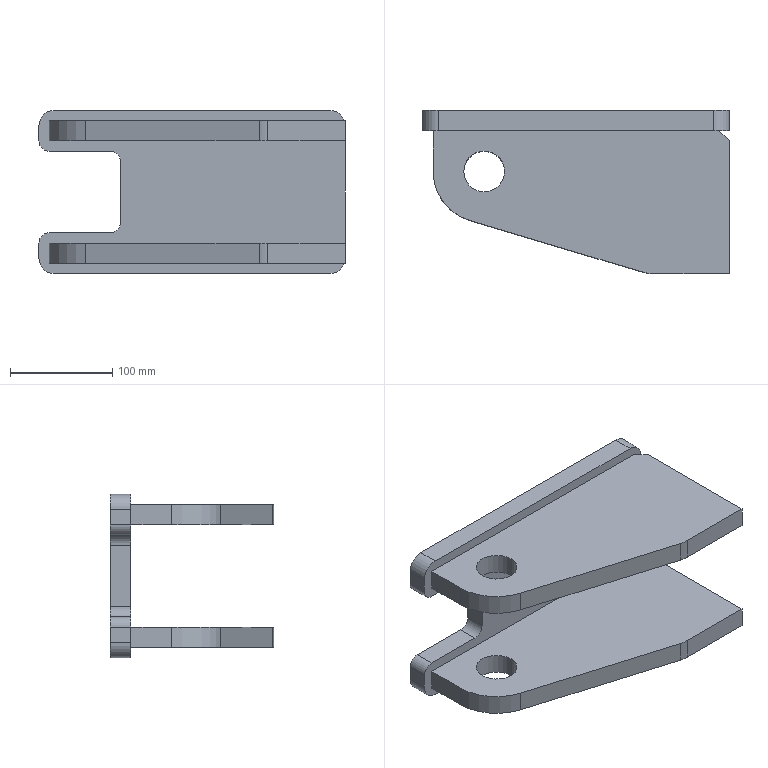Part | SolidWorks | features BaseBody 3 | 3 solids | 42 faces | box 300 x 160 x 160 mm | volume 2125789 mm3 | plane 26 | cylinder 16 | commonest cylinder face diameters 20 x4 30 x4 40 x4 60 x2 100 x2
STEP:
#1=CARTESIAN_POINT('',(-150.,-10.,-65.));
#2=VERTEX_POINT('',#1);
#3=CARTESIAN_POINT('',(-150.,-10.,-50.));
#4=VERTEX_POINT('',#3);
#5=CARTESIAN_POINT('',(-150.,-10.,-65.));
#6=DIRECTION('',(0.,0.,1.));
#7=VECTOR('',#6,1000.);
#8=LINE('',#5,#7);
#9=EDGE_CURVE('',#2,#4,#8,.T.);
#10=ORIENTED_EDGE('',*,*,#9,.T.);
#11=CARTESIAN_POINT('',(-150.,10.,-50.));
#12=VERTEX_POINT('',#11);
#13=CARTESIAN_POINT('',(-150.,10.,-50.));
#14=DIRECTION('',(0.,1.,0.));
#15=VECTOR('',#14,1000.);
#16=LINE('',#13,#15);
#17=EDGE_CURVE('',#4,#12,#16,.T.);
#18=ORIENTED_EDGE('',*,*,#17,.T.);
#19=CARTESIAN_POINT('',(-150.,10.,-65.));
#20=VERTEX_POINT('',#19);
#21=CARTESIAN_POINT('',(-150.,10.,-65.));
#22=DIRECTION('',(0.,0.,1.));
#23=VECTOR('',#22,1000.);
#24=LINE('',#21,#23);
#25=EDGE_CURVE('',#20,#12,#24,.T.);
#26=ORIENTED_EDGE('',*,*,#25,.F.);
#27=CARTESIAN_POINT('',(-150.,10.,-65.));
#28=DIRECTION('',(0.,-1.,0.));
#29=VECTOR('',#28,1000.);
#30=LINE('',#27,#29);
#31=EDGE_CURVE('',#20,#2,#30,.T.);
#32=ORIENTED_EDGE('',*,*,#31,.T.);
#33=EDGE_LOOP('',(#10,#18,#26,#32));
#34=FACE_OUTER_BOUND('',#33,.T.);
#35=CARTESIAN_POINT('',(-150.,10.,-65.));
#36=DIRECTION('',(1.,0.,0.));
#37=DIRECTION('',(0.,0.,-1.));
#38=AXIS2_PLACEMENT_3D('',#35,#36,#37);
#39=PLANE('',#38);
#40=ADVANCED_FACE('',(#34),#39,.F.);
#41=CARTESIAN_POINT('',(-150.,-10.,65.));
#42=VERTEX_POINT('',#41);
#43=CARTESIAN_POINT('',(-135.,-10.,80.));
#44=VERTEX_POINT('',#43);
#45=CARTESIAN_POINT('',(-135.,-10.,65.));
#46=DIRECTION('',(0.,1.,0.));
#47=DIRECTION('',(0.,0.,1.));
#48=AXIS2_PLACEMENT_3D('',#45,#46,#47);
#49=CIRCLE('',#48,15.);
#50=EDGE_CURVE('',#42,#44,#49,.T.);
#51=ORIENTED_EDGE('',*,*,#50,.T.);
#52=CARTESIAN_POINT('',(-135.,10.,80.));
#53=VERTEX_POINT('',#52);
#54=CARTESIAN_POINT('',(-135.,10.,80.));
#55=DIRECTION('',(0.,-1.,0.));
#56=VECTOR('',#55,1000.);
#57=LINE('',#54,#56);
#58=EDGE_CURVE('',#53,#44,#57,.T.);
#59=ORIENTED_EDGE('',*,*,#58,.F.);
#60=CARTESIAN_POINT('',(-150.,10.,65.));
#61=VERTEX_POINT('',#60);
#62=CARTESIAN_POINT('',(-135.,10.,65.));
#63=DIRECTION('',(0.,1.,0.));
#64=DIRECTION('',(0.,0.,1.));
#65=AXIS2_PLACEMENT_3D('',#62,#63,#64);
#66=CIRCLE('',#65,15.);
#67=EDGE_CURVE('',#61,#53,#66,.T.);
#68=ORIENTED_EDGE('',*,*,#67,.F.);
#69=CARTESIAN_POINT('',(-150.,10.,65.));
#70=DIRECTION('',(0.,-1.,0.));
#71=VECTOR('',#70,1000.);
#72=LINE('',#69,#71);
#73=EDGE_CURVE('',#61,#42,#72,.T.);
#74=ORIENTED_EDGE('',*,*,#73,.T.);
#75=EDGE_LOOP('',(#51,#59,#68,#74));
#76=FACE_OUTER_BOUND('',#75,.T.);
#77=CARTESIAN_POINT('',(-135.,10.,65.));
#78=DIRECTION('',(0.,-1.,0.));
#79=DIRECTION('',(0.,0.,-1.));
#80=AXIS2_PLACEMENT_3D('',#77,#78,#79);
#81=CYLINDRICAL_SURFACE('',#80,15.);
#82=ADVANCED_FACE('',(#76),#81,.T.);
#83=CARTESIAN_POINT('',(135.,-10.,80.));
#84=VERTEX_POINT('',#83);
#85=CARTESIAN_POINT('',(-135.,-10.,80.));
#86=DIRECTION('',(1.,0.,0.));
#87=VECTOR('',#86,1000.);
#88=LINE('',#85,#87);
#89=EDGE_CURVE('',#44,#84,#88,.T.);
#90=ORIENTED_EDGE('',*,*,#89,.T.);
#91=CARTESIAN_POINT('',(135.,10.,80.));
#92=VERTEX_POINT('',#91);
#93=CARTESIAN_POINT('',(135.,10.,80.));
#94=DIRECTION('',(0.,-1.,0.));
#95=VECTOR('',#94,1000.);
#96=LINE('',#93,#95);
#97=EDGE_CURVE('',#92,#84,#96,.T.);
#98=ORIENTED_EDGE('',*,*,#97,.F.);
#99=CARTESIAN_POINT('',(-135.,10.,80.));
#100=DIRECTION('',(1.,0.,0.));
#101=VECTOR('',#100,1000.);
#102=LINE('',#99,#101);
#103=EDGE_CURVE('',#53,#92,#102,.T.);
#104=ORIENTED_EDGE('',*,*,#103,.F.);
#105=ORIENTED_EDGE('',*,*,#58,.T.);
#106=EDGE_LOOP('',(#90,#98,#104,#105));
#107=FACE_OUTER_BOUND('',#106,.T.);
#108=CARTESIAN_POINT('',(-135.,10.,80.));
#109=DIRECTION('',(0.,0.,-1.));
#110=DIRECTION('',(-1.,0.,0.));
#111=AXIS2_PLACEMENT_3D('',#108,#109,#110);
#112=PLANE('',#111);
#113=ADVANCED_FACE('',(#107),#112,.F.);
#114=CARTESIAN_POINT('',(150.,-10.,65.));
#115=VERTEX_POINT('',#114);
#116=CARTESIAN_POINT('',(135.,-10.,65.));
#117=DIRECTION('',(0.,1.,0.));
#118=DIRECTION('',(0.,0.,1.));
#119=AXIS2_PLACEMENT_3D('',#116,#117,#118);
#120=CIRCLE('',#119,15.);
#121=EDGE_CURVE('',#84,#115,#120,.T.);
#122=ORIENTED_EDGE('',*,*,#121,.T.);
#123=CARTESIAN_POINT('',(150.,10.,65.));
#124=VERTEX_POINT('',#123);
#125=CARTESIAN_POINT('',(150.,10.,65.));
#126=DIRECTION('',(0.,-1.,0.));
#127=VECTOR('',#126,1000.);
#128=LINE('',#125,#127);
#129=EDGE_CURVE('',#124,#115,#128,.T.);
#130=ORIENTED_EDGE('',*,*,#129,.F.);
#131=CARTESIAN_POINT('',(135.,10.,65.));
#132=DIRECTION('',(0.,1.,0.));
#133=DIRECTION('',(0.,0.,1.));
#134=AXIS2_PLACEMENT_3D('',#131,#132,#133);
#135=CIRCLE('',#134,15.);
#136=EDGE_CURVE('',#92,#124,#135,.T.);
#137=ORIENTED_EDGE('',*,*,#136,.F.);
#138=ORIENTED_EDGE('',*,*,#97,.T.);
#139=EDGE_LOOP('',(#122,#130,#137,#138));
#140=FACE_OUTER_BOUND('',#139,.T.);
#141=CARTESIAN_POINT('',(135.,10.,65.));
#142=DIRECTION('',(0.,-1.,0.));
#143=DIRECTION('',(0.,0.,-1.));
#144=AXIS2_PLACEMENT_3D('',#141,#142,#143);
#145=CYLINDRICAL_SURFACE('',#144,15.);
#146=ADVANCED_FACE('',(#140),#145,.T.);
#147=CARTESIAN_POINT('',(150.,-10.,-65.));
#148=VERTEX_POINT('',#147);
#149=CARTESIAN_POINT('',(150.,-10.,-65.));
#150=DIRECTION('',(0.,0.,-1.));
#151=VECTOR('',#150,1000.);
#152=LINE('',#149,#151);
#153=EDGE_CURVE('',#115,#148,#152,.T.);
#154=ORIENTED_EDGE('',*,*,#153,.T.);
#155=CARTESIAN_POINT('',(150.,10.,-65.));
#156=VERTEX_POINT('',#155);
#157=CARTESIAN_POINT('',(150.,10.,-65.));
#158=DIRECTION('',(0.,-1.,0.));
#159=VECTOR('',#158,1000.);
#160=LINE('',#157,#159);
#161=EDGE_CURVE('',#156,#148,#160,.T.);
#162=ORIENTED_EDGE('',*,*,#161,.F.);
#163=CARTESIAN_POINT('',(150.,10.,-65.));
#164=DIRECTION('',(0.,0.,-1.));
#165=VECTOR('',#164,1000.);
#166=LINE('',#163,#165);
#167=EDGE_CURVE('',#124,#156,#166,.T.);
#168=ORIENTED_EDGE('',*,*,#167,.F.);
#169=ORIENTED_EDGE('',*,*,#129,.T.);
#170=EDGE_LOOP('',(#154,#162,#168,#169));
#171=FACE_OUTER_BOUND('',#170,.T.);
#172=CARTESIAN_POINT('',(150.,10.,-65.));
#173=DIRECTION('',(-1.,0.,0.));
#174=DIRECTION('',(0.,0.,1.));
#175=AXIS2_PLACEMENT_3D('',#172,#173,#174);
#176=PLANE('',#175);
#177=ADVANCED_FACE('',(#171),#176,.F.);
#178=CARTESIAN_POINT('',(135.,-10.,-80.));
#179=VERTEX_POINT('',#178);
#180=CARTESIAN_POINT('',(135.,-10.,-65.));
#181=DIRECTION('',(0.,1.,0.));
#182=DIRECTION('',(0.,0.,-1.));
#183=AXIS2_PLACEMENT_3D('',#180,#181,#182);
#184=CIRCLE('',#183,15.);
#185=EDGE_CURVE('',#148,#179,#184,.T.);
#186=ORIENTED_EDGE('',*,*,#185,.T.);
#187=CARTESIAN_POINT('',(135.,10.,-80.));
#188=VERTEX_POINT('',#187);
#189=CARTESIAN_POINT('',(135.,10.,-80.));
#190=DIRECTION('',(0.,-1.,0.));
#191=VECTOR('',#190,1000.);
#192=LINE('',#189,#191);
#193=EDGE_CURVE('',#188,#179,#192,.T.);
#194=ORIENTED_EDGE('',*,*,#193,.F.);
#195=CARTESIAN_POINT('',(135.,10.,-65.));
#196=DIRECTION('',(0.,1.,0.));
#197=DIRECTION('',(0.,0.,-1.));
#198=AXIS2_PLACEMENT_3D('',#195,#196,#197);
#199=CIRCLE('',#198,15.);
#200=EDGE_CURVE('',#156,#188,#199,.T.);
#201=ORIENTED_EDGE('',*,*,#200,.F.);
#202=ORIENTED_EDGE('',*,*,#161,.T.);
#203=EDGE_LOOP('',(#186,#194,#201,#202));
#204=FACE_OUTER_BOUND('',#203,.T.);
#205=CARTESIAN_POINT('',(135.,10.,-65.));
#206=DIRECTION('',(0.,-1.,0.));
#207=DIRECTION('',(0.,0.,-1.));
#208=AXIS2_PLACEMENT_3D('',#205,#206,#207);
#209=CYLINDRICAL_SURFACE('',#208,15.);
#210=ADVANCED_FACE('',(#204),#209,.T.);
#211=CARTESIAN_POINT('',(-135.,-10.,-80.));
#212=VERTEX_POINT('',#211);
#213=CARTESIAN_POINT('',(-135.,-10.,-80.));
#214=DIRECTION('',(-1.,0.,0.));
#215=VECTOR('',#214,1000.);
#216=LINE('',#213,#215);
#217=EDGE_CURVE('',#179,#212,#216,.T.);
#218=ORIENTED_EDGE('',*,*,#217,.T.);
#219=CARTESIAN_POINT('',(-135.,10.,-80.));
#220=VERTEX_POINT('',#219);
#221=CARTESIAN_POINT('',(-135.,10.,-80.));
#222=DIRECTION('',(0.,-1.,0.));
#223=VECTOR('',#222,1000.);
#224=LINE('',#221,#223);
#225=EDGE_CURVE('',#220,#212,#224,.T.);
#226=ORIENTED_EDGE('',*,*,#225,.F.);
#227=CARTESIAN_POINT('',(-135.,10.,-80.));
#228=DIRECTION('',(-1.,0.,0.));
#229=VECTOR('',#228,1000.);
#230=LINE('',#227,#229);
#231=EDGE_CURVE('',#188,#220,#230,.T.);
#232=ORIENTED_EDGE('',*,*,#231,.F.);
#233=ORIENTED_EDGE('',*,*,#193,.T.);
#234=EDGE_LOOP('',(#218,#226,#232,#233));
#235=FACE_OUTER_BOUND('',#234,.T.);
#236=CARTESIAN_POINT('',(-135.,10.,-80.));
#237=DIRECTION('',(0.,0.,1.));
#238=DIRECTION('',(1.,0.,0.));
#239=AXIS2_PLACEMENT_3D('',#236,#237,#238);
#240=PLANE('',#239);
#241=ADVANCED_FACE('',(#235),#240,.F.);
#242=CARTESIAN_POINT('',(-135.,-10.,-65.));
#243=DIRECTION('',(0.,1.,0.));
#244=DIRECTION('',(0.,0.,1.));
#245=AXIS2_PLACEMENT_3D('',#242,#243,#244);
#246=CIRCLE('',#245,15.);
#247=EDGE_CURVE('',#212,#2,#246,.T.);
#248=ORIENTED_EDGE('',*,*,#247,.T.);
#249=ORIENTED_EDGE('',*,*,#31,.F.);
#250=CARTESIAN_POINT('',(-135.,10.,-65.));
#251=DIRECTION('',(0.,1.,0.));
#252=DIRECTION('',(0.,0.,1.));
#253=AXIS2_PLACEMENT_3D('',#250,#251,#252);
#254=CIRCLE('',#253,15.);
#255=EDGE_CURVE('',#220,#20,#254,.T.);
#256=ORIENTED_EDGE('',*,*,#255,.F.);
#257=ORIENTED_EDGE('',*,*,#225,.T.);
#258=EDGE_LOOP('',(#248,#249,#256,#257));
#259=FACE_OUTER_BOUND('',#258,.T.);
#260=CARTESIAN_POINT('',(-135.,10.,-65.));
#261=DIRECTION('',(0.,-1.,0.));
#262=DIRECTION('',(0.,0.,-1.));
#263=AXIS2_PLACEMENT_3D('',#260,#261,#262);
#264=CYLINDRICAL_SURFACE('',#263,15.);
#265=ADVANCED_FACE('',(#259),#264,.T.);
#266=CARTESIAN_POINT('',(-150.,10.,50.));
#267=VERTEX_POINT('',#266);
#268=CARTESIAN_POINT('',(-150.,10.,-65.));
#269=DIRECTION('',(0.,0.,1.));
#270=VECTOR('',#269,1000.);
#271=LINE('',#268,#270);
#272=EDGE_CURVE('',#267,#61,#271,.T.);
#273=ORIENTED_EDGE('',*,*,#272,.F.);
#274=CARTESIAN_POINT('',(-150.,-10.,50.));
#275=VERTEX_POINT('',#274);
#276=CARTESIAN_POINT('',(-150.,10.,50.));
#277=DIRECTION('',(0.,-1.,0.));
#278=VECTOR('',#277,1000.);
#279=LINE('',#276,#278);
#280=EDGE_CURVE('',#267,#275,#279,.T.);
#281=ORIENTED_EDGE('',*,*,#280,.T.);
#282=CARTESIAN_POINT('',(-150.,-10.,-65.));
#283=DIRECTION('',(0.,0.,1.));
#284=VECTOR('',#283,1000.);
#285=LINE('',#282,#284);
#286=EDGE_CURVE('',#275,#42,#285,.T.);
#287=ORIENTED_EDGE('',*,*,#286,.T.);
#288=ORIENTED_EDGE('',*,*,#73,.F.);
#289=EDGE_LOOP('',(#273,#281,#287,#288));
#290=FACE_OUTER_BOUND('',#289,.T.);
#291=CARTESIAN_POINT('',(-150.,10.,-65.));
#292=DIRECTION('',(1.,0.,0.));
#293=DIRECTION('',(0.,0.,-1.));
#294=AXIS2_PLACEMENT_3D('',#291,#292,#293);
#295=PLANE('',#294);
#296=ADVANCED_FACE('',(#290),#295,.F.);
#297=CARTESIAN_POINT('',(-140.,10.,40.));
#298=VERTEX_POINT('',#297);
#299=CARTESIAN_POINT('',(-80.,10.,40.));
#300=VERTEX_POINT('',#299);
#301=CARTESIAN_POINT('',(-150.,10.,40.));
#302=DIRECTION('',(1.,0.,0.));
#303=VECTOR('',#302,1000.);
#304=LINE('',#301,#303);
#305=EDGE_CURVE('',#298,#300,#304,.T.);
#306=ORIENTED_EDGE('',*,*,#305,.F.);
#307=CARTESIAN_POINT('',(-140.,10.,50.));
#308=DIRECTION('',(0.,1.,0.));
#309=DIRECTION('',(0.,0.,1.));
#310=AXIS2_PLACEMENT_3D('',#307,#308,#309);
#311=CIRCLE('',#310,10.);
#312=EDGE_CURVE('',#298,#267,#311,.T.);
#313=ORIENTED_EDGE('',*,*,#312,.T.);
#314=ORIENTED_EDGE('',*,*,#272,.T.);
#315=ORIENTED_EDGE('',*,*,#67,.T.);
#316=ORIENTED_EDGE('',*,*,#103,.T.);
#317=ORIENTED_EDGE('',*,*,#136,.T.);
#318=ORIENTED_EDGE('',*,*,#167,.T.);
#319=ORIENTED_EDGE('',*,*,#200,.T.);
#320=ORIENTED_EDGE('',*,*,#231,.T.);
#321=ORIENTED_EDGE('',*,*,#255,.T.);
#322=ORIENTED_EDGE('',*,*,#25,.T.);
#323=CARTESIAN_POINT('',(-140.,10.,-40.));
#324=VERTEX_POINT('',#323);
#325=CARTESIAN_POINT('',(-140.,10.,-50.));
#326=DIRECTION('',(0.,1.,0.));
#327=DIRECTION('',(0.,0.,1.));
#328=AXIS2_PLACEMENT_3D('',#325,#326,#327);
#329=CIRCLE('',#328,10.);
#330=EDGE_CURVE('',#12,#324,#329,.T.);
#331=ORIENTED_EDGE('',*,*,#330,.T.);
#332=CARTESIAN_POINT('',(-80.,10.,-40.));
#333=VERTEX_POINT('',#332);
#334=CARTESIAN_POINT('',(-150.,10.,-40.));
#335=DIRECTION('',(-1.,0.,0.));
#336=VECTOR('',#335,1000.);
#337=LINE('',#334,#336);
#338=EDGE_CURVE('',#333,#324,#337,.T.);
#339=ORIENTED_EDGE('',*,*,#338,.F.);
#340=CARTESIAN_POINT('',(-70.,10.,-30.));
#341=VERTEX_POINT('',#340);
#342=CARTESIAN_POINT('',(-80.,10.,-30.));
#343=DIRECTION('',(0.,1.,0.));
#344=DIRECTION('',(0.,0.,-1.));
#345=AXIS2_PLACEMENT_3D('',#342,#343,#344);
#346=CIRCLE('',#345,10.);
#347=EDGE_CURVE('',#341,#333,#346,.T.);
#348=ORIENTED_EDGE('',*,*,#347,.F.);
#349=CARTESIAN_POINT('',(-70.,10.,30.));
#350=VERTEX_POINT('',#349);
#351=CARTESIAN_POINT('',(-70.,10.,-30.));
#352=DIRECTION('',(0.,0.,-1.));
#353=VECTOR('',#352,1000.);
#354=LINE('',#351,#353);
#355=EDGE_CURVE('',#350,#341,#354,.T.);
#356=ORIENTED_EDGE('',*,*,#355,.F.);
#357=CARTESIAN_POINT('',(-80.,10.,30.));
#358=DIRECTION('',(0.,1.,0.));
#359=DIRECTION('',(0.,0.,1.));
#360=AXIS2_PLACEMENT_3D('',#357,#358,#359);
#361=CIRCLE('',#360,10.);
#362=EDGE_CURVE('',#300,#350,#361,.T.);
#363=ORIENTED_EDGE('',*,*,#362,.F.);
#364=EDGE_LOOP('',(#306,#313,#314,#315,#316,#317,#318,#319,#320,#321,#322,#331,#339,#348,#356,#363));
#365=FACE_OUTER_BOUND('',#364,.T.);
#366=CARTESIAN_POINT('',(-135.,10.,65.));
#367=DIRECTION('',(0.,1.,0.));
#368=DIRECTION('',(0.,0.,1.));
#369=AXIS2_PLACEMENT_3D('',#366,#367,#368);
#370=PLANE('',#369);
#371=ADVANCED_FACE('',(#365),#370,.T.);
#372=ORIENTED_EDGE('',*,*,#286,.F.);
#373=CARTESIAN_POINT('',(-140.,-10.,40.));
#374=VERTEX_POINT('',#373);
#375=CARTESIAN_POINT('',(-140.,-10.,50.));
#376=DIRECTION('',(0.,-1.,0.));
#377=DIRECTION('',(0.,0.,1.));
#378=AXIS2_PLACEMENT_3D('',#375,#376,#377);
#379=CIRCLE('',#378,10.);
#380=EDGE_CURVE('',#275,#374,#379,.T.);
#381=ORIENTED_EDGE('',*,*,#380,.T.);
#382=CARTESIAN_POINT('',(-80.,-10.,40.));
#383=VERTEX_POINT('',#382);
#384=CARTESIAN_POINT('',(-150.,-10.,40.));
#385=DIRECTION('',(1.,0.,0.));
#386=VECTOR('',#385,1000.);
#387=LINE('',#384,#386);
#388=EDGE_CURVE('',#374,#383,#387,.T.);
#389=ORIENTED_EDGE('',*,*,#388,.T.);
#390=CARTESIAN_POINT('',(-70.,-10.,30.));
#391=VERTEX_POINT('',#390);
#392=CARTESIAN_POINT('',(-80.,-10.,30.));
#393=DIRECTION('',(0.,1.,0.));
#394=DIRECTION('',(0.,0.,1.));
#395=AXIS2_PLACEMENT_3D('',#392,#393,#394);
#396=CIRCLE('',#395,10.);
#397=EDGE_CURVE('',#383,#391,#396,.T.);
#398=ORIENTED_EDGE('',*,*,#397,.T.);
#399=CARTESIAN_POINT('',(-70.,-10.,-30.));
#400=VERTEX_POINT('',#399);
#401=CARTESIAN_POINT('',(-70.,-10.,-30.));
#402=DIRECTION('',(0.,0.,-1.));
#403=VECTOR('',#402,1000.);
#404=LINE('',#401,#403);
#405=EDGE_CURVE('',#391,#400,#404,.T.);
#406=ORIENTED_EDGE('',*,*,#405,.T.);
#407=CARTESIAN_POINT('',(-80.,-10.,-40.));
#408=VERTEX_POINT('',#407);
#409=CARTESIAN_POINT('',(-80.,-10.,-30.));
#410=DIRECTION('',(0.,1.,0.));
#411=DIRECTION('',(0.,0.,-1.));
#412=AXIS2_PLACEMENT_3D('',#409,#410,#411);
#413=CIRCLE('',#412,10.);
#414=EDGE_CURVE('',#400,#408,#413,.T.);
#415=ORIENTED_EDGE('',*,*,#414,.T.);
#416=CARTESIAN_POINT('',(-140.,-10.,-40.));
#417=VERTEX_POINT('',#416);
#418=CARTESIAN_POINT('',(-150.,-10.,-40.));
#419=DIRECTION('',(-1.,0.,0.));
#420=VECTOR('',#419,1000.);
#421=LINE('',#418,#420);
#422=EDGE_CURVE('',#408,#417,#421,.T.);
#423=ORIENTED_EDGE('',*,*,#422,.T.);
#424=CARTESIAN_POINT('',(-140.,-10.,-50.));
#425=DIRECTION('',(0.,-1.,0.));
#426=DIRECTION('',(0.,0.,1.));
#427=AXIS2_PLACEMENT_3D('',#424,#425,#426);
#428=CIRCLE('',#427,10.);
#429=EDGE_CURVE('',#417,#4,#428,.T.);
#430=ORIENTED_EDGE('',*,*,#429,.T.);
#431=ORIENTED_EDGE('',*,*,#9,.F.);
#432=ORIENTED_EDGE('',*,*,#247,.F.);
#433=ORIENTED_EDGE('',*,*,#217,.F.);
#434=ORIENTED_EDGE('',*,*,#185,.F.);
#435=ORIENTED_EDGE('',*,*,#153,.F.);
#436=ORIENTED_EDGE('',*,*,#121,.F.);
#437=ORIENTED_EDGE('',*,*,#89,.F.);
#438=ORIENTED_EDGE('',*,*,#50,.F.);
#439=EDGE_LOOP('',(#372,#381,#389,#398,#406,#415,#423,#430,#431,#432,#433,#434,#435,#436,#437,#438));
#440=FACE_OUTER_BOUND('',#439,.T.);
#441=CARTESIAN_POINT('',(-135.,-10.,65.));
#442=DIRECTION('',(0.,1.,0.));
#443=DIRECTION('',(0.,0.,1.));
#444=AXIS2_PLACEMENT_3D('',#441,#442,#443);
#445=PLANE('',#444);
#446=ADVANCED_FACE('',(#440),#445,.F.);
#447=ORIENTED_EDGE('',*,*,#338,.T.);
#448=CARTESIAN_POINT('',(-140.,-10.,-40.));
#449=DIRECTION('',(0.,-1.,0.));
#450=VECTOR('',#449,1000.);
#451=LINE('',#448,#450);
#452=EDGE_CURVE('',#324,#417,#451,.T.);
#453=ORIENTED_EDGE('',*,*,#452,.T.);
#454=ORIENTED_EDGE('',*,*,#422,.F.);
#455=CARTESIAN_POINT('',(-80.,-10.,-40.));
#456=DIRECTION('',(0.,1.,0.));
#457=VECTOR('',#456,1000.);
#458=LINE('',#455,#457);
#459=EDGE_CURVE('',#408,#333,#458,.T.);
#460=ORIENTED_EDGE('',*,*,#459,.T.);
#461=EDGE_LOOP('',(#447,#453,#454,#460));
#462=FACE_OUTER_BOUND('',#461,.T.);
#463=CARTESIAN_POINT('',(-150.,-10.,-40.));
#464=DIRECTION('',(0.,0.,-1.));
#465=DIRECTION('',(-1.,0.,0.));
#466=AXIS2_PLACEMENT_3D('',#463,#464,#465);
#467=PLANE('',#466);
#468=ADVANCED_FACE('',(#462),#467,.F.);
#469=ORIENTED_EDGE('',*,*,#347,.T.);
#470=ORIENTED_EDGE('',*,*,#459,.F.);
#471=ORIENTED_EDGE('',*,*,#414,.F.);
#472=CARTESIAN_POINT('',(-70.,-10.,-30.));
#473=DIRECTION('',(0.,1.,0.));
#474=VECTOR('',#473,1000.);
#475=LINE('',#472,#474);
#476=EDGE_CURVE('',#400,#341,#475,.T.);
#477=ORIENTED_EDGE('',*,*,#476,.T.);
#478=EDGE_LOOP('',(#469,#470,#471,#477));
#479=FACE_OUTER_BOUND('',#478,.T.);
#480=CARTESIAN_POINT('',(-80.,-10.,-30.));
#481=DIRECTION('',(0.,1.,0.));
#482=DIRECTION('',(0.,0.,1.));
#483=AXIS2_PLACEMENT_3D('',#480,#481,#482);
#484=CYLINDRICAL_SURFACE('',#483,10.);
#485=ADVANCED_FACE('',(#479),#484,.F.);
#486=ORIENTED_EDGE('',*,*,#355,.T.);
#487=ORIENTED_EDGE('',*,*,#476,.F.);
#488=ORIENTED_EDGE('',*,*,#405,.F.);
#489=CARTESIAN_POINT('',(-70.,-10.,30.));
#490=DIRECTION('',(0.,1.,0.));
#491=VECTOR('',#490,1000.);
#492=LINE('',#489,#491);
#493=EDGE_CURVE('',#391,#350,#492,.T.);
#494=ORIENTED_EDGE('',*,*,#493,.T.);
#495=EDGE_LOOP('',(#486,#487,#488,#494));
#496=FACE_OUTER_BOUND('',#495,.T.);
#497=CARTESIAN_POINT('',(-70.,-10.,-30.));
#498=DIRECTION('',(1.,0.,0.));
#499=DIRECTION('',(0.,0.,-1.));
#500=AXIS2_PLACEMENT_3D('',#497,#498,#499);
#501=PLANE('',#500);
#502=ADVANCED_FACE('',(#496),#501,.F.);
#503=ORIENTED_EDGE('',*,*,#362,.T.);
#504=ORIENTED_EDGE('',*,*,#493,.F.);
#505=ORIENTED_EDGE('',*,*,#397,.F.);
#506=CARTESIAN_POINT('',(-80.,-10.,40.));
#507=DIRECTION('',(0.,1.,0.));
#508=VECTOR('',#507,1000.);
#509=LINE('',#506,#508);
#510=EDGE_CURVE('',#383,#300,#509,.T.);
#511=ORIENTED_EDGE('',*,*,#510,.T.);
#512=EDGE_LOOP('',(#503,#504,#505,#511));
#513=FACE_OUTER_BOUND('',#512,.T.);
#514=CARTESIAN_POINT('',(-80.,-10.,30.));
#515=DIRECTION('',(0.,1.,0.));
#516=DIRECTION('',(0.,0.,1.));
#517=AXIS2_PLACEMENT_3D('',#514,#515,#516);
#518=CYLINDRICAL_SURFACE('',#517,10.);
#519=ADVANCED_FACE('',(#513),#518,.F.);
#520=ORIENTED_EDGE('',*,*,#388,.F.);
#521=CARTESIAN_POINT('',(-140.,-10.,40.));
#522=DIRECTION('',(0.,1.,0.));
#523=VECTOR('',#522,1000.);
#524=LINE('',#521,#523);
#525=EDGE_CURVE('',#374,#298,#524,.T.);
#526=ORIENTED_EDGE('',*,*,#525,.T.);
#527=ORIENTED_EDGE('',*,*,#305,.T.);
#528=ORIENTED_EDGE('',*,*,#510,.F.);
#529=EDGE_LOOP('',(#520,#526,#527,#528));
#530=FACE_OUTER_BOUND('',#529,.T.);
#531=CARTESIAN_POINT('',(-150.,-10.,40.));
#532=DIRECTION('',(0.,0.,1.));
#533=DIRECTION('',(1.,0.,0.));
#534=AXIS2_PLACEMENT_3D('',#531,#532,#533);
#535=PLANE('',#534);
#536=ADVANCED_FACE('',(#530),#535,.F.);
#537=ORIENTED_EDGE('',*,*,#380,.F.);
#538=ORIENTED_EDGE('',*,*,#280,.F.);
#539=ORIENTED_EDGE('',*,*,#312,.F.);
#540=ORIENTED_EDGE('',*,*,#525,.F.);
#541=EDGE_LOOP('',(#537,#538,#539,#540));
#542=FACE_OUTER_BOUND('',#541,.T.);
#543=CARTESIAN_POINT('',(-140.,-10.,50.));
#544=DIRECTION('',(0.,1.,0.));
#545=DIRECTION('',(0.,0.,1.));
#546=AXIS2_PLACEMENT_3D('',#543,#544,#545);
#547=CYLINDRICAL_SURFACE('',#546,10.);
#548=ADVANCED_FACE('',(#542),#547,.T.);
#549=ORIENTED_EDGE('',*,*,#429,.F.);
#550=ORIENTED_EDGE('',*,*,#452,.F.);
#551=ORIENTED_EDGE('',*,*,#330,.F.);
#552=ORIENTED_EDGE('',*,*,#17,.F.);
#553=EDGE_LOOP('',(#549,#550,#551,#552));
#554=FACE_OUTER_BOUND('',#553,.T.);
#555=CARTESIAN_POINT('',(-140.,10.,-50.));
#556=DIRECTION('',(0.,1.,0.));
#557=DIRECTION('',(0.,0.,1.));
#558=AXIS2_PLACEMENT_3D('',#555,#556,#557);
#559=CYLINDRICAL_SURFACE('',#558,10.);
#560=ADVANCED_FACE('',(#554),#559,.T.);
#561=CLOSED_SHELL('',(#40,#82,#113,#146,#177,#210,#241,#265,#296,#371,#446,#468,#485,#502,#519,#536,#548,#560));
#562=MANIFOLD_SOLID_BREP('',#561);
#563=CARTESIAN_POINT('',(-110.,-50.,70.));
#564=VERTEX_POINT('',#563);
#565=CARTESIAN_POINT('',(-70.,-50.,70.));
#566=VERTEX_POINT('',#565);
#567=CARTESIAN_POINT('',(-90.,-50.,70.));
#568=DIRECTION('',(0.,0.,1.));
#569=DIRECTION('',(1.,0.,0.));
#570=AXIS2_PLACEMENT_3D('',#567,#568,#569);
#571=CIRCLE('',#570,20.);
#572=EDGE_CURVE('',#564,#566,#571,.T.);
#573=ORIENTED_EDGE('',*,*,#572,.T.);
#574=CARTESIAN_POINT('',(-70.,-50.,50.));
#575=VERTEX_POINT('',#574);
#576=CARTESIAN_POINT('',(-70.,-50.,70.));
#577=DIRECTION('',(0.,0.,-1.));
#578=VECTOR('',#577,1000.);
#579=LINE('',#576,#578);
#580=EDGE_CURVE('',#566,#575,#579,.T.);
#581=ORIENTED_EDGE('',*,*,#580,.T.);
#582=CARTESIAN_POINT('',(-110.,-50.,50.));
#583=VERTEX_POINT('',#582);
#584=CARTESIAN_POINT('',(-90.,-50.,50.));
#585=DIRECTION('',(0.,0.,1.));
#586=DIRECTION('',(1.,0.,0.));
#587=AXIS2_PLACEMENT_3D('',#584,#585,#586);
#588=CIRCLE('',#587,20.);
#589=EDGE_CURVE('',#583,#575,#588,.T.);
#590=ORIENTED_EDGE('',*,*,#589,.F.);
#591=CARTESIAN_POINT('',(-110.,-50.,70.));
#592=DIRECTION('',(0.,0.,-1.));
#593=VECTOR('',#592,1000.);
#594=LINE('',#591,#593);
#595=EDGE_CURVE('',#564,#583,#594,.T.);
#596=ORIENTED_EDGE('',*,*,#595,.F.);
#597=EDGE_LOOP('',(#573,#581,#590,#596));
#598=FACE_OUTER_BOUND('',#597,.T.);
#599=CARTESIAN_POINT('',(-90.,-50.,70.));
#600=DIRECTION('',(0.,0.,-1.));
#601=DIRECTION('',(-1.,0.,0.));
#602=AXIS2_PLACEMENT_3D('',#599,#600,#601);
#603=CYLINDRICAL_SURFACE('',#602,20.);
#604=ADVANCED_FACE('',(#598),#603,.F.);
#605=CARTESIAN_POINT('',(74.387,-150.,70.));
#606=VERTEX_POINT('',#605);
#607=CARTESIAN_POINT('',(150.,-150.,70.));
#608=VERTEX_POINT('',#607);
#609=CARTESIAN_POINT('',(150.,-150.,70.));
#610=DIRECTION('',(1.,0.,0.));
#611=VECTOR('',#610,1000.);
#612=LINE('',#609,#611);
#613=EDGE_CURVE('',#606,#608,#612,.T.);
#614=ORIENTED_EDGE('',*,*,#613,.T.);
#615=CARTESIAN_POINT('',(150.,-20.,70.));
#616=VERTEX_POINT('',#615);
#617=CARTESIAN_POINT('',(150.,-20.,70.));
#618=DIRECTION('',(0.,1.,0.));
#619=VECTOR('',#618,1000.);
#620=LINE('',#617,#619);
#621=EDGE_CURVE('',#608,#616,#620,.T.);
#622=ORIENTED_EDGE('',*,*,#621,.T.);
#623=CARTESIAN_POINT('',(140.,-10.,70.));
#624=VERTEX_POINT('',#623);
#625=CARTESIAN_POINT('',(140.,-10.,70.));
#626=DIRECTION('',(-0.7071,0.7071,0.));
#627=VECTOR('',#626,1000.);
#628=LINE('',#625,#627);
#629=EDGE_CURVE('',#616,#624,#628,.T.);
#630=ORIENTED_EDGE('',*,*,#629,.T.);
#631=CARTESIAN_POINT('',(-140.,-10.,70.));
#632=VERTEX_POINT('',#631);
#633=CARTESIAN_POINT('',(-140.,-10.,70.));
#634=DIRECTION('',(-1.,0.,0.));
#635=VECTOR('',#634,1000.);
#636=LINE('',#633,#635);
#637=EDGE_CURVE('',#624,#632,#636,.T.);
#638=ORIENTED_EDGE('',*,*,#637,.T.);
#639=CARTESIAN_POINT('',(-140.,-50.,70.));
#640=VERTEX_POINT('',#639);
#641=CARTESIAN_POINT('',(-140.,-50.,70.));
#642=DIRECTION('',(0.,-1.,0.));
#643=VECTOR('',#642,1000.);
#644=LINE('',#641,#643);
#645=EDGE_CURVE('',#632,#640,#644,.T.);
#646=ORIENTED_EDGE('',*,*,#645,.T.);
#647=CARTESIAN_POINT('',(-104.317,-97.907,70.));
#648=VERTEX_POINT('',#647);
#649=CARTESIAN_POINT('',(-90.,-50.,70.));
#650=DIRECTION('',(0.,0.,1.));
#651=DIRECTION('',(1.,0.,0.));
#652=AXIS2_PLACEMENT_3D('',#649,#650,#651);
#653=CIRCLE('',#652,50.);
#654=EDGE_CURVE('',#640,#648,#653,.T.);
#655=ORIENTED_EDGE('',*,*,#654,.T.);
#656=CARTESIAN_POINT('',(65.797,-148.744,70.));
#657=VERTEX_POINT('',#656);
#658=CARTESIAN_POINT('',(65.797,-148.744,70.));
#659=DIRECTION('',(0.9581,-0.2863,0.));
#660=VECTOR('',#659,1000.);
#661=LINE('',#658,#660);
#662=EDGE_CURVE('',#648,#657,#661,.T.);
#663=ORIENTED_EDGE('',*,*,#662,.T.);
#664=CARTESIAN_POINT('',(74.387,-120.,70.));
#665=DIRECTION('',(0.,0.,1.));
#666=DIRECTION('',(-1.,0.,0.));
#667=AXIS2_PLACEMENT_3D('',#664,#665,#666);
#668=CIRCLE('',#667,30.);
#669=EDGE_CURVE('',#657,#606,#668,.T.);
#670=ORIENTED_EDGE('',*,*,#669,.T.);
#671=EDGE_LOOP('',(#614,#622,#630,#638,#646,#655,#663,#670));
#672=FACE_OUTER_BOUND('',#671,.T.);
#673=ORIENTED_EDGE('',*,*,#572,.F.);
#674=CARTESIAN_POINT('',(-90.,-50.,70.));
#675=DIRECTION('',(0.,0.,1.));
#676=DIRECTION('',(1.,0.,0.));
#677=AXIS2_PLACEMENT_3D('',#674,#675,#676);
#678=CIRCLE('',#677,20.);
#679=EDGE_CURVE('',#566,#564,#678,.T.);
#680=ORIENTED_EDGE('',*,*,#679,.F.);
#681=EDGE_LOOP('',(#673,#680));
#682=FACE_BOUND('',#681,.T.);
#683=CARTESIAN_POINT('',(74.387,-120.,70.));
#684=DIRECTION('',(0.,0.,-1.));
#685=DIRECTION('',(-1.,0.,0.));
#686=AXIS2_PLACEMENT_3D('',#683,#684,#685);
#687=PLANE('',#686);
#688=ADVANCED_FACE('',(#672,#682),#687,.F.);
#689=CARTESIAN_POINT('',(74.387,-150.,50.));
#690=VERTEX_POINT('',#689);
#691=CARTESIAN_POINT('',(150.,-150.,50.));
#692=VERTEX_POINT('',#691);
#693=CARTESIAN_POINT('',(150.,-150.,50.));
#694=DIRECTION('',(1.,0.,0.));
#695=VECTOR('',#694,1000.);
#696=LINE('',#693,#695);
#697=EDGE_CURVE('',#690,#692,#696,.T.);
#698=ORIENTED_EDGE('',*,*,#697,.F.);
#699=CARTESIAN_POINT('',(65.797,-148.744,50.));
#700=VERTEX_POINT('',#699);
#701=CARTESIAN_POINT('',(74.387,-120.,50.));
#702=DIRECTION('',(0.,0.,1.));
#703=DIRECTION('',(-1.,0.,0.));
#704=AXIS2_PLACEMENT_3D('',#701,#702,#703);
#705=CIRCLE('',#704,30.);
#706=EDGE_CURVE('',#700,#690,#705,.T.);
#707=ORIENTED_EDGE('',*,*,#706,.F.);
#708=CARTESIAN_POINT('',(-104.317,-97.907,50.));
#709=VERTEX_POINT('',#708);
#710=CARTESIAN_POINT('',(65.797,-148.744,50.));
#711=DIRECTION('',(0.9581,-0.2863,0.));
#712=VECTOR('',#711,1000.);
#713=LINE('',#710,#712);
#714=EDGE_CURVE('',#709,#700,#713,.T.);
#715=ORIENTED_EDGE('',*,*,#714,.F.);
#716=CARTESIAN_POINT('',(-140.,-50.,50.));
#717=VERTEX_POINT('',#716);
#718=CARTESIAN_POINT('',(-90.,-50.,50.));
#719=DIRECTION('',(0.,0.,1.));
#720=DIRECTION('',(1.,0.,0.));
#721=AXIS2_PLACEMENT_3D('',#718,#719,#720);
#722=CIRCLE('',#721,50.);
#723=EDGE_CURVE('',#717,#709,#722,.T.);
#724=ORIENTED_EDGE('',*,*,#723,.F.);
#725=CARTESIAN_POINT('',(-140.,-10.,50.));
#726=VERTEX_POINT('',#725);
#727=CARTESIAN_POINT('',(-140.,-50.,50.));
#728=DIRECTION('',(0.,-1.,0.));
#729=VECTOR('',#728,1000.);
#730=LINE('',#727,#729);
#731=EDGE_CURVE('',#726,#717,#730,.T.);
#732=ORIENTED_EDGE('',*,*,#731,.F.);
#733=CARTESIAN_POINT('',(140.,-10.,50.));
#734=VERTEX_POINT('',#733);
#735=CARTESIAN_POINT('',(-140.,-10.,50.));
#736=DIRECTION('',(-1.,0.,0.));
#737=VECTOR('',#736,1000.);
#738=LINE('',#735,#737);
#739=EDGE_CURVE('',#734,#726,#738,.T.);
#740=ORIENTED_EDGE('',*,*,#739,.F.);
#741=CARTESIAN_POINT('',(150.,-20.,50.));
#742=VERTEX_POINT('',#741);
#743=CARTESIAN_POINT('',(140.,-10.,50.));
#744=DIRECTION('',(-0.7071,0.7071,0.));
#745=VECTOR('',#744,1000.);
#746=LINE('',#743,#745);
#747=EDGE_CURVE('',#742,#734,#746,.T.);
#748=ORIENTED_EDGE('',*,*,#747,.F.);
#749=CARTESIAN_POINT('',(150.,-20.,50.));
#750=DIRECTION('',(0.,1.,0.));
#751=VECTOR('',#750,1000.);
#752=LINE('',#749,#751);
#753=EDGE_CURVE('',#692,#742,#752,.T.);
#754=ORIENTED_EDGE('',*,*,#753,.F.);
#755=EDGE_LOOP('',(#698,#707,#715,#724,#732,#740,#748,#754));
#756=FACE_OUTER_BOUND('',#755,.T.);
#757=ORIENTED_EDGE('',*,*,#589,.T.);
#758=CARTESIAN_POINT('',(-90.,-50.,50.));
#759=DIRECTION('',(0.,0.,1.));
#760=DIRECTION('',(1.,0.,0.));
#761=AXIS2_PLACEMENT_3D('',#758,#759,#760);
#762=CIRCLE('',#761,20.);
#763=EDGE_CURVE('',#575,#583,#762,.T.);
#764=ORIENTED_EDGE('',*,*,#763,.T.);
#765=EDGE_LOOP('',(#757,#764));
#766=FACE_BOUND('',#765,.T.);
#767=CARTESIAN_POINT('',(74.387,-120.,50.));
#768=DIRECTION('',(0.,0.,-1.));
#769=DIRECTION('',(-1.,0.,0.));
#770=AXIS2_PLACEMENT_3D('',#767,#768,#769);
#771=PLANE('',#770);
#772=ADVANCED_FACE('',(#756,#766),#771,.T.);
#773=ORIENTED_EDGE('',*,*,#697,.T.);
#774=CARTESIAN_POINT('',(150.,-150.,70.));
#775=DIRECTION('',(0.,0.,-1.));
#776=VECTOR('',#775,1000.);
#777=LINE('',#774,#776);
#778=EDGE_CURVE('',#608,#692,#777,.T.);
#779=ORIENTED_EDGE('',*,*,#778,.F.);
#780=ORIENTED_EDGE('',*,*,#613,.F.);
#781=CARTESIAN_POINT('',(74.387,-150.,70.));
#782=DIRECTION('',(0.,0.,-1.));
#783=VECTOR('',#782,1000.);
#784=LINE('',#781,#783);
#785=EDGE_CURVE('',#606,#690,#784,.T.);
#786=ORIENTED_EDGE('',*,*,#785,.T.);
#787=EDGE_LOOP('',(#773,#779,#780,#786));
#788=FACE_OUTER_BOUND('',#787,.T.);
#789=CARTESIAN_POINT('',(150.,-150.,70.));
#790=DIRECTION('',(0.,1.,0.));
#791=DIRECTION('',(0.,0.,1.));
#792=AXIS2_PLACEMENT_3D('',#789,#790,#791);
#793=PLANE('',#792);
#794=ADVANCED_FACE('',(#788),#793,.F.);
#795=ORIENTED_EDGE('',*,*,#753,.T.);
#796=CARTESIAN_POINT('',(150.,-20.,70.));
#797=DIRECTION('',(0.,0.,-1.));
#798=VECTOR('',#797,1000.);
#799=LINE('',#796,#798);
#800=EDGE_CURVE('',#616,#742,#799,.T.);
#801=ORIENTED_EDGE('',*,*,#800,.F.);
#802=ORIENTED_EDGE('',*,*,#621,.F.);
#803=ORIENTED_EDGE('',*,*,#778,.T.);
#804=EDGE_LOOP('',(#795,#801,#802,#803));
#805=FACE_OUTER_BOUND('',#804,.T.);
#806=CARTESIAN_POINT('',(150.,-20.,70.));
#807=DIRECTION('',(-1.,0.,0.));
#808=DIRECTION('',(0.,-1.,0.));
#809=AXIS2_PLACEMENT_3D('',#806,#807,#808);
#810=PLANE('',#809);
#811=ADVANCED_FACE('',(#805),#810,.F.);
#812=ORIENTED_EDGE('',*,*,#747,.T.);
#813=CARTESIAN_POINT('',(140.,-10.,70.));
#814=DIRECTION('',(0.,0.,-1.));
#815=VECTOR('',#814,1000.);
#816=LINE('',#813,#815);
#817=EDGE_CURVE('',#624,#734,#816,.T.);
#818=ORIENTED_EDGE('',*,*,#817,.F.);
#819=ORIENTED_EDGE('',*,*,#629,.F.);
#820=ORIENTED_EDGE('',*,*,#800,.T.);
#821=EDGE_LOOP('',(#812,#818,#819,#820));
#822=FACE_OUTER_BOUND('',#821,.T.);
#823=CARTESIAN_POINT('',(140.,-10.,70.));
#824=DIRECTION('',(-0.7071,-0.7071,0.));
#825=DIRECTION('',(0.7071,-0.7071,0.));
#826=AXIS2_PLACEMENT_3D('',#823,#824,#825);
#827=PLANE('',#826);
#828=ADVANCED_FACE('',(#822),#827,.F.);
#829=ORIENTED_EDGE('',*,*,#739,.T.);
#830=CARTESIAN_POINT('',(-140.,-10.,70.));
#831=DIRECTION('',(0.,0.,-1.));
#832=VECTOR('',#831,1000.);
#833=LINE('',#830,#832);
#834=EDGE_CURVE('',#632,#726,#833,.T.);
#835=ORIENTED_EDGE('',*,*,#834,.F.);
#836=ORIENTED_EDGE('',*,*,#637,.F.);
#837=ORIENTED_EDGE('',*,*,#817,.T.);
#838=EDGE_LOOP('',(#829,#835,#836,#837));
#839=FACE_OUTER_BOUND('',#838,.T.);
#840=CARTESIAN_POINT('',(-140.,-10.,70.));
#841=DIRECTION('',(0.,-1.,0.));
#842=DIRECTION('',(1.,0.,0.));
#843=AXIS2_PLACEMENT_3D('',#840,#841,#842);
#844=PLANE('',#843);
#845=ADVANCED_FACE('',(#839),#844,.F.);
#846=ORIENTED_EDGE('',*,*,#731,.T.);
#847=CARTESIAN_POINT('',(-140.,-50.,70.));
#848=DIRECTION('',(0.,0.,-1.));
#849=VECTOR('',#848,1000.);
#850=LINE('',#847,#849);
#851=EDGE_CURVE('',#640,#717,#850,.T.);
#852=ORIENTED_EDGE('',*,*,#851,.F.);
#853=ORIENTED_EDGE('',*,*,#645,.F.);
#854=ORIENTED_EDGE('',*,*,#834,.T.);
#855=EDGE_LOOP('',(#846,#852,#853,#854));
#856=FACE_OUTER_BOUND('',#855,.T.);
#857=CARTESIAN_POINT('',(-140.,-50.,70.));
#858=DIRECTION('',(1.,0.,0.));
#859=DIRECTION('',(0.,0.,-1.));
#860=AXIS2_PLACEMENT_3D('',#857,#858,#859);
#861=PLANE('',#860);
#862=ADVANCED_FACE('',(#856),#861,.F.);
#863=ORIENTED_EDGE('',*,*,#723,.T.);
#864=CARTESIAN_POINT('',(-104.317,-97.907,70.));
#865=DIRECTION('',(0.,0.,-1.));
#866=VECTOR('',#865,1000.);
#867=LINE('',#864,#866);
#868=EDGE_CURVE('',#648,#709,#867,.T.);
#869=ORIENTED_EDGE('',*,*,#868,.F.);
#870=ORIENTED_EDGE('',*,*,#654,.F.);
#871=ORIENTED_EDGE('',*,*,#851,.T.);
#872=EDGE_LOOP('',(#863,#869,#870,#871));
#873=FACE_OUTER_BOUND('',#872,.T.);
#874=CARTESIAN_POINT('',(-90.,-50.,70.));
#875=DIRECTION('',(0.,0.,-1.));
#876=DIRECTION('',(-1.,0.,0.));
#877=AXIS2_PLACEMENT_3D('',#874,#875,#876);
#878=CYLINDRICAL_SURFACE('',#877,50.);
#879=ADVANCED_FACE('',(#873),#878,.T.);
#880=ORIENTED_EDGE('',*,*,#714,.T.);
#881=CARTESIAN_POINT('',(65.797,-148.744,70.));
#882=DIRECTION('',(0.,0.,-1.));
#883=VECTOR('',#882,1000.);
#884=LINE('',#881,#883);
#885=EDGE_CURVE('',#657,#700,#884,.T.);
#886=ORIENTED_EDGE('',*,*,#885,.F.);
#887=ORIENTED_EDGE('',*,*,#662,.F.);
#888=ORIENTED_EDGE('',*,*,#868,.T.);
#889=EDGE_LOOP('',(#880,#886,#887,#888));
#890=FACE_OUTER_BOUND('',#889,.T.);
#891=CARTESIAN_POINT('',(65.797,-148.744,70.));
#892=DIRECTION('',(0.2863,0.9581,0.));
#893=DIRECTION('',(-0.9581,0.2863,0.));
#894=AXIS2_PLACEMENT_3D('',#891,#892,#893);
#895=PLANE('',#894);
#896=ADVANCED_FACE('',(#890),#895,.F.);
#897=ORIENTED_EDGE('',*,*,#706,.T.);
#898=ORIENTED_EDGE('',*,*,#785,.F.);
#899=ORIENTED_EDGE('',*,*,#669,.F.);
#900=ORIENTED_EDGE('',*,*,#885,.T.);
#901=EDGE_LOOP('',(#897,#898,#899,#900));
#902=FACE_OUTER_BOUND('',#901,.T.);
#903=CARTESIAN_POINT('',(74.387,-120.,70.));
#904=DIRECTION('',(0.,0.,-1.));
#905=DIRECTION('',(-1.,0.,0.));
#906=AXIS2_PLACEMENT_3D('',#903,#904,#905);
#907=CYLINDRICAL_SURFACE('',#906,30.);
#908=ADVANCED_FACE('',(#902),#907,.T.);
#909=ORIENTED_EDGE('',*,*,#580,.F.);
#910=ORIENTED_EDGE('',*,*,#679,.T.);
#911=ORIENTED_EDGE('',*,*,#595,.T.);
#912=ORIENTED_EDGE('',*,*,#763,.F.);
#913=EDGE_LOOP('',(#909,#910,#911,#912));
#914=FACE_OUTER_BOUND('',#913,.T.);
#915=CARTESIAN_POINT('',(-90.,-50.,70.));
#916=DIRECTION('',(0.,0.,-1.));
#917=DIRECTION('',(-1.,0.,0.));
#918=AXIS2_PLACEMENT_3D('',#915,#916,#917);
#919=CYLINDRICAL_SURFACE('',#918,20.);
#920=ADVANCED_FACE('',(#914),#919,.F.);
#921=CLOSED_SHELL('',(#604,#688,#772,#794,#811,#828,#845,#862,#879,#896,#908,#920));
#922=MANIFOLD_SOLID_BREP('',#921);
#923=CARTESIAN_POINT('',(-70.,-50.,-70.));
#924=VERTEX_POINT('',#923);
#925=CARTESIAN_POINT('',(-110.,-50.,-70.));
#926=VERTEX_POINT('',#925);
#927=CARTESIAN_POINT('',(-90.,-50.,-70.));
#928=DIRECTION('',(0.,0.,1.));
#929=DIRECTION('',(1.,0.,0.));
#930=AXIS2_PLACEMENT_3D('',#927,#928,#929);
#931=CIRCLE('',#930,20.);
#932=EDGE_CURVE('',#924,#926,#931,.T.);
#933=ORIENTED_EDGE('',*,*,#932,.F.);
#934=CARTESIAN_POINT('',(-70.,-50.,-50.));
#935=VERTEX_POINT('',#934);
#936=CARTESIAN_POINT('',(-70.,-50.,-70.));
#937=DIRECTION('',(0.,0.,1.));
#938=VECTOR('',#937,1000.);
#939=LINE('',#936,#938);
#940=EDGE_CURVE('',#924,#935,#939,.T.);
#941=ORIENTED_EDGE('',*,*,#940,.T.);
#942=CARTESIAN_POINT('',(-110.,-50.,-50.));
#943=VERTEX_POINT('',#942);
#944=CARTESIAN_POINT('',(-90.,-50.,-50.));
#945=DIRECTION('',(0.,0.,1.));
#946=DIRECTION('',(1.,0.,0.));
#947=AXIS2_PLACEMENT_3D('',#944,#945,#946);
#948=CIRCLE('',#947,20.);
#949=EDGE_CURVE('',#935,#943,#948,.T.);
#950=ORIENTED_EDGE('',*,*,#949,.T.);
#951=CARTESIAN_POINT('',(-110.,-50.,-70.));
#952=DIRECTION('',(0.,0.,1.));
#953=VECTOR('',#952,1000.);
#954=LINE('',#951,#953);
#955=EDGE_CURVE('',#926,#943,#954,.T.);
#956=ORIENTED_EDGE('',*,*,#955,.F.);
#957=EDGE_LOOP('',(#933,#941,#950,#956));
#958=FACE_OUTER_BOUND('',#957,.T.);
#959=CARTESIAN_POINT('',(-90.,-50.,-70.));
#960=DIRECTION('',(0.,0.,1.));
#961=DIRECTION('',(-1.,0.,0.));
#962=AXIS2_PLACEMENT_3D('',#959,#960,#961);
#963=CYLINDRICAL_SURFACE('',#962,20.);
#964=ADVANCED_FACE('',(#958),#963,.F.);
#965=CARTESIAN_POINT('',(74.387,-150.,-70.));
#966=VERTEX_POINT('',#965);
#967=CARTESIAN_POINT('',(150.,-150.,-70.));
#968=VERTEX_POINT('',#967);
#969=CARTESIAN_POINT('',(150.,-150.,-70.));
#970=DIRECTION('',(1.,0.,0.));
#971=VECTOR('',#970,1000.);
#972=LINE('',#969,#971);
#973=EDGE_CURVE('',#966,#968,#972,.T.);
#974=ORIENTED_EDGE('',*,*,#973,.F.);
#975=CARTESIAN_POINT('',(65.797,-148.744,-70.));
#976=VERTEX_POINT('',#975);
#977=CARTESIAN_POINT('',(74.387,-120.,-70.));
#978=DIRECTION('',(0.,0.,1.));
#979=DIRECTION('',(-1.,0.,0.));
#980=AXIS2_PLACEMENT_3D('',#977,#978,#979);
#981=CIRCLE('',#980,30.);
#982=EDGE_CURVE('',#976,#966,#981,.T.);
#983=ORIENTED_EDGE('',*,*,#982,.F.);
#984=CARTESIAN_POINT('',(-104.317,-97.907,-70.));
#985=VERTEX_POINT('',#984);
#986=CARTESIAN_POINT('',(65.797,-148.744,-70.));
#987=DIRECTION('',(0.9581,-0.2863,0.));
#988=VECTOR('',#987,1000.);
#989=LINE('',#986,#988);
#990=EDGE_CURVE('',#985,#976,#989,.T.);
#991=ORIENTED_EDGE('',*,*,#990,.F.);
#992=CARTESIAN_POINT('',(-140.,-50.,-70.));
#993=VERTEX_POINT('',#992);
#994=CARTESIAN_POINT('',(-90.,-50.,-70.));
#995=DIRECTION('',(0.,0.,1.));
#996=DIRECTION('',(1.,0.,0.));
#997=AXIS2_PLACEMENT_3D('',#994,#995,#996);
#998=CIRCLE('',#997,50.);
#999=EDGE_CURVE('',#993,#985,#998,.T.);
#1000=ORIENTED_EDGE('',*,*,#999,.F.);
#1001=CARTESIAN_POINT('',(-140.,-10.,-70.));
#1002=VERTEX_POINT('',#1001);
#1003=CARTESIAN_POINT('',(-140.,-50.,-70.));
#1004=DIRECTION('',(0.,-1.,0.));
#1005=VECTOR('',#1004,1000.);
#1006=LINE('',#1003,#1005);
#1007=EDGE_CURVE('',#1002,#993,#1006,.T.);
#1008=ORIENTED_EDGE('',*,*,#1007,.F.);
#1009=CARTESIAN_POINT('',(140.,-10.,-70.));
#1010=VERTEX_POINT('',#1009);
#1011=CARTESIAN_POINT('',(-140.,-10.,-70.));
#1012=DIRECTION('',(-1.,0.,0.));
#1013=VECTOR('',#1012,1000.);
#1014=LINE('',#1011,#1013);
#1015=EDGE_CURVE('',#1010,#1002,#1014,.T.);
#1016=ORIENTED_EDGE('',*,*,#1015,.F.);
#1017=CARTESIAN_POINT('',(150.,-20.,-70.));
#1018=VERTEX_POINT('',#1017);
#1019=CARTESIAN_POINT('',(140.,-10.,-70.));
#1020=DIRECTION('',(-0.7071,0.7071,0.));
#1021=VECTOR('',#1020,1000.);
#1022=LINE('',#1019,#1021);
#1023=EDGE_CURVE('',#1018,#1010,#1022,.T.);
#1024=ORIENTED_EDGE('',*,*,#1023,.F.);
#1025=CARTESIAN_POINT('',(150.,-20.,-70.));
#1026=DIRECTION('',(0.,1.,0.));
#1027=VECTOR('',#1026,1000.);
#1028=LINE('',#1025,#1027);
#1029=EDGE_CURVE('',#968,#1018,#1028,.T.);
#1030=ORIENTED_EDGE('',*,*,#1029,.F.);
#1031=EDGE_LOOP('',(#974,#983,#991,#1000,#1008,#1016,#1024,#1030));
#1032=FACE_OUTER_BOUND('',#1031,.T.);
#1033=CARTESIAN_POINT('',(-90.,-50.,-70.));
#1034=DIRECTION('',(0.,0.,1.));
#1035=DIRECTION('',(1.,0.,0.));
#1036=AXIS2_PLACEMENT_3D('',#1033,#1034,#1035);
#1037=CIRCLE('',#1036,20.);
#1038=EDGE_CURVE('',#926,#924,#1037,.T.);
#1039=ORIENTED_EDGE('',*,*,#1038,.T.);
#1040=ORIENTED_EDGE('',*,*,#932,.T.);
#1041=EDGE_LOOP('',(#1039,#1040));
#1042=FACE_BOUND('',#1041,.T.);
#1043=CARTESIAN_POINT('',(74.387,-120.,-70.));
#1044=DIRECTION('',(0.,0.,1.));
#1045=DIRECTION('',(-1.,0.,0.));
#1046=AXIS2_PLACEMENT_3D('',#1043,#1044,#1045);
#1047=PLANE('',#1046);
#1048=ADVANCED_FACE('',(#1032,#1042),#1047,.F.);
#1049=CARTESIAN_POINT('',(74.387,-150.,-50.));
#1050=VERTEX_POINT('',#1049);
#1051=CARTESIAN_POINT('',(150.,-150.,-50.));
#1052=VERTEX_POINT('',#1051);
#1053=CARTESIAN_POINT('',(150.,-150.,-50.));
#1054=DIRECTION('',(1.,0.,0.));
#1055=VECTOR('',#1054,1000.);
#1056=LINE('',#1053,#1055);
#1057=EDGE_CURVE('',#1050,#1052,#1056,.T.);
#1058=ORIENTED_EDGE('',*,*,#1057,.T.);
#1059=CARTESIAN_POINT('',(150.,-20.,-50.));
#1060=VERTEX_POINT('',#1059);
#1061=CARTESIAN_POINT('',(150.,-20.,-50.));
#1062=DIRECTION('',(0.,1.,0.));
#1063=VECTOR('',#1062,1000.);
#1064=LINE('',#1061,#1063);
#1065=EDGE_CURVE('',#1052,#1060,#1064,.T.);
#1066=ORIENTED_EDGE('',*,*,#1065,.T.);
#1067=CARTESIAN_POINT('',(140.,-10.,-50.));
#1068=VERTEX_POINT('',#1067);
#1069=CARTESIAN_POINT('',(140.,-10.,-50.));
#1070=DIRECTION('',(-0.7071,0.7071,0.));
#1071=VECTOR('',#1070,1000.);
#1072=LINE('',#1069,#1071);
#1073=EDGE_CURVE('',#1060,#1068,#1072,.T.);
#1074=ORIENTED_EDGE('',*,*,#1073,.T.);
#1075=CARTESIAN_POINT('',(-140.,-10.,-50.));
#1076=VERTEX_POINT('',#1075);
#1077=CARTESIAN_POINT('',(-140.,-10.,-50.));
#1078=DIRECTION('',(-1.,0.,0.));
#1079=VECTOR('',#1078,1000.);
#1080=LINE('',#1077,#1079);
#1081=EDGE_CURVE('',#1068,#1076,#1080,.T.);
#1082=ORIENTED_EDGE('',*,*,#1081,.T.);
#1083=CARTESIAN_POINT('',(-140.,-50.,-50.));
#1084=VERTEX_POINT('',#1083);
#1085=CARTESIAN_POINT('',(-140.,-50.,-50.));
#1086=DIRECTION('',(0.,-1.,0.));
#1087=VECTOR('',#1086,1000.);
#1088=LINE('',#1085,#1087);
#1089=EDGE_CURVE('',#1076,#1084,#1088,.T.);
#1090=ORIENTED_EDGE('',*,*,#1089,.T.);
#1091=CARTESIAN_POINT('',(-104.317,-97.907,-50.));
#1092=VERTEX_POINT('',#1091);
#1093=CARTESIAN_POINT('',(-90.,-50.,-50.));
#1094=DIRECTION('',(0.,0.,1.));
#1095=DIRECTION('',(1.,0.,0.));
#1096=AXIS2_PLACEMENT_3D('',#1093,#1094,#1095);
#1097=CIRCLE('',#1096,50.);
#1098=EDGE_CURVE('',#1084,#1092,#1097,.T.);
#1099=ORIENTED_EDGE('',*,*,#1098,.T.);
#1100=CARTESIAN_POINT('',(65.797,-148.744,-50.));
#1101=VERTEX_POINT('',#1100);
#1102=CARTESIAN_POINT('',(65.797,-148.744,-50.));
#1103=DIRECTION('',(0.9581,-0.2863,0.));
#1104=VECTOR('',#1103,1000.);
#1105=LINE('',#1102,#1104);
#1106=EDGE_CURVE('',#1092,#1101,#1105,.T.);
#1107=ORIENTED_EDGE('',*,*,#1106,.T.);
#1108=CARTESIAN_POINT('',(74.387,-120.,-50.));
#1109=DIRECTION('',(0.,0.,1.));
#1110=DIRECTION('',(-1.,0.,0.));
#1111=AXIS2_PLACEMENT_3D('',#1108,#1109,#1110);
#1112=CIRCLE('',#1111,30.);
#1113=EDGE_CURVE('',#1101,#1050,#1112,.T.);
#1114=ORIENTED_EDGE('',*,*,#1113,.T.);
#1115=EDGE_LOOP('',(#1058,#1066,#1074,#1082,#1090,#1099,#1107,#1114));
#1116=FACE_OUTER_BOUND('',#1115,.T.);
#1117=CARTESIAN_POINT('',(-90.,-50.,-50.));
#1118=DIRECTION('',(0.,0.,1.));
#1119=DIRECTION('',(1.,0.,0.));
#1120=AXIS2_PLACEMENT_3D('',#1117,#1118,#1119);
#1121=CIRCLE('',#1120,20.);
#1122=EDGE_CURVE('',#943,#935,#1121,.T.);
#1123=ORIENTED_EDGE('',*,*,#1122,.F.);
#1124=ORIENTED_EDGE('',*,*,#949,.F.);
#1125=EDGE_LOOP('',(#1123,#1124));
#1126=FACE_BOUND('',#1125,.T.);
#1127=CARTESIAN_POINT('',(74.387,-120.,-50.));
#1128=DIRECTION('',(0.,0.,1.));
#1129=DIRECTION('',(-1.,0.,0.));
#1130=AXIS2_PLACEMENT_3D('',#1127,#1128,#1129);
#1131=PLANE('',#1130);
#1132=ADVANCED_FACE('',(#1116,#1126),#1131,.T.);
#1133=ORIENTED_EDGE('',*,*,#1057,.F.);
#1134=CARTESIAN_POINT('',(74.387,-150.,-70.));
#1135=DIRECTION('',(0.,0.,1.));
#1136=VECTOR('',#1135,1000.);
#1137=LINE('',#1134,#1136);
#1138=EDGE_CURVE('',#966,#1050,#1137,.T.);
#1139=ORIENTED_EDGE('',*,*,#1138,.F.);
#1140=ORIENTED_EDGE('',*,*,#973,.T.);
#1141=CARTESIAN_POINT('',(150.,-150.,-70.));
#1142=DIRECTION('',(0.,0.,1.));
#1143=VECTOR('',#1142,1000.);
#1144=LINE('',#1141,#1143);
#1145=EDGE_CURVE('',#968,#1052,#1144,.T.);
#1146=ORIENTED_EDGE('',*,*,#1145,.T.);
#1147=EDGE_LOOP('',(#1133,#1139,#1140,#1146));
#1148=FACE_OUTER_BOUND('',#1147,.T.);
#1149=CARTESIAN_POINT('',(150.,-150.,-70.));
#1150=DIRECTION('',(0.,1.,0.));
#1151=DIRECTION('',(0.,0.,-1.));
#1152=AXIS2_PLACEMENT_3D('',#1149,#1150,#1151);
#1153=PLANE('',#1152);
#1154=ADVANCED_FACE('',(#1148),#1153,.F.);
#1155=ORIENTED_EDGE('',*,*,#1065,.F.);
#1156=ORIENTED_EDGE('',*,*,#1145,.F.);
#1157=ORIENTED_EDGE('',*,*,#1029,.T.);
#1158=CARTESIAN_POINT('',(150.,-20.,-70.));
#1159=DIRECTION('',(0.,0.,1.));
#1160=VECTOR('',#1159,1000.);
#1161=LINE('',#1158,#1160);
#1162=EDGE_CURVE('',#1018,#1060,#1161,.T.);
#1163=ORIENTED_EDGE('',*,*,#1162,.T.);
#1164=EDGE_LOOP('',(#1155,#1156,#1157,#1163));
#1165=FACE_OUTER_BOUND('',#1164,.T.);
#1166=CARTESIAN_POINT('',(150.,-20.,-70.));
#1167=DIRECTION('',(-1.,0.,0.));
#1168=DIRECTION('',(0.,-1.,0.));
#1169=AXIS2_PLACEMENT_3D('',#1166,#1167,#1168);
#1170=PLANE('',#1169);
#1171=ADVANCED_FACE('',(#1165),#1170,.F.);
#1172=ORIENTED_EDGE('',*,*,#1073,.F.);
#1173=ORIENTED_EDGE('',*,*,#1162,.F.);
#1174=ORIENTED_EDGE('',*,*,#1023,.T.);
#1175=CARTESIAN_POINT('',(140.,-10.,-70.));
#1176=DIRECTION('',(0.,0.,1.));
#1177=VECTOR('',#1176,1000.);
#1178=LINE('',#1175,#1177);
#1179=EDGE_CURVE('',#1010,#1068,#1178,.T.);
#1180=ORIENTED_EDGE('',*,*,#1179,.T.);
#1181=EDGE_LOOP('',(#1172,#1173,#1174,#1180));
#1182=FACE_OUTER_BOUND('',#1181,.T.);
#1183=CARTESIAN_POINT('',(140.,-10.,-70.));
#1184=DIRECTION('',(-0.7071,-0.7071,0.));
#1185=DIRECTION('',(0.7071,-0.7071,0.));
#1186=AXIS2_PLACEMENT_3D('',#1183,#1184,#1185);
#1187=PLANE('',#1186);
#1188=ADVANCED_FACE('',(#1182),#1187,.F.);
#1189=ORIENTED_EDGE('',*,*,#1081,.F.);
#1190=ORIENTED_EDGE('',*,*,#1179,.F.);
#1191=ORIENTED_EDGE('',*,*,#1015,.T.);
#1192=CARTESIAN_POINT('',(-140.,-10.,-70.));
#1193=DIRECTION('',(0.,0.,1.));
#1194=VECTOR('',#1193,1000.);
#1195=LINE('',#1192,#1194);
#1196=EDGE_CURVE('',#1002,#1076,#1195,.T.);
#1197=ORIENTED_EDGE('',*,*,#1196,.T.);
#1198=EDGE_LOOP('',(#1189,#1190,#1191,#1197));
#1199=FACE_OUTER_BOUND('',#1198,.T.);
#1200=CARTESIAN_POINT('',(-140.,-10.,-70.));
#1201=DIRECTION('',(0.,-1.,0.));
#1202=DIRECTION('',(1.,0.,0.));
#1203=AXIS2_PLACEMENT_3D('',#1200,#1201,#1202);
#1204=PLANE('',#1203);
#1205=ADVANCED_FACE('',(#1199),#1204,.F.);
#1206=ORIENTED_EDGE('',*,*,#1089,.F.);
#1207=ORIENTED_EDGE('',*,*,#1196,.F.);
#1208=ORIENTED_EDGE('',*,*,#1007,.T.);
#1209=CARTESIAN_POINT('',(-140.,-50.,-70.));
#1210=DIRECTION('',(0.,0.,1.));
#1211=VECTOR('',#1210,1000.);
#1212=LINE('',#1209,#1211);
#1213=EDGE_CURVE('',#993,#1084,#1212,.T.);
#1214=ORIENTED_EDGE('',*,*,#1213,.T.);
#1215=EDGE_LOOP('',(#1206,#1207,#1208,#1214));
#1216=FACE_OUTER_BOUND('',#1215,.T.);
#1217=CARTESIAN_POINT('',(-140.,-50.,-70.));
#1218=DIRECTION('',(1.,0.,0.));
#1219=DIRECTION('',(0.,0.,1.));
#1220=AXIS2_PLACEMENT_3D('',#1217,#1218,#1219);
#1221=PLANE('',#1220);
#1222=ADVANCED_FACE('',(#1216),#1221,.F.);
#1223=ORIENTED_EDGE('',*,*,#1098,.F.);
#1224=ORIENTED_EDGE('',*,*,#1213,.F.);
#1225=ORIENTED_EDGE('',*,*,#999,.T.);
#1226=CARTESIAN_POINT('',(-104.317,-97.907,-70.));
#1227=DIRECTION('',(0.,0.,1.));
#1228=VECTOR('',#1227,1000.);
#1229=LINE('',#1226,#1228);
#1230=EDGE_CURVE('',#985,#1092,#1229,.T.);
#1231=ORIENTED_EDGE('',*,*,#1230,.T.);
#1232=EDGE_LOOP('',(#1223,#1224,#1225,#1231));
#1233=FACE_OUTER_BOUND('',#1232,.T.);
#1234=CARTESIAN_POINT('',(-90.,-50.,-70.));
#1235=DIRECTION('',(0.,0.,1.));
#1236=DIRECTION('',(-1.,0.,0.));
#1237=AXIS2_PLACEMENT_3D('',#1234,#1235,#1236);
#1238=CYLINDRICAL_SURFACE('',#1237,50.);
#1239=ADVANCED_FACE('',(#1233),#1238,.T.);
#1240=ORIENTED_EDGE('',*,*,#1106,.F.);
#1241=ORIENTED_EDGE('',*,*,#1230,.F.);
#1242=ORIENTED_EDGE('',*,*,#990,.T.);
#1243=CARTESIAN_POINT('',(65.797,-148.744,-70.));
#1244=DIRECTION('',(0.,0.,1.));
#1245=VECTOR('',#1244,1000.);
#1246=LINE('',#1243,#1245);
#1247=EDGE_CURVE('',#976,#1101,#1246,.T.);
#1248=ORIENTED_EDGE('',*,*,#1247,.T.);
#1249=EDGE_LOOP('',(#1240,#1241,#1242,#1248));
#1250=FACE_OUTER_BOUND('',#1249,.T.);
#1251=CARTESIAN_POINT('',(65.797,-148.744,-70.));
#1252=DIRECTION('',(0.2863,0.9581,0.));
#1253=DIRECTION('',(-0.9581,0.2863,0.));
#1254=AXIS2_PLACEMENT_3D('',#1251,#1252,#1253);
#1255=PLANE('',#1254);
#1256=ADVANCED_FACE('',(#1250),#1255,.F.);
#1257=ORIENTED_EDGE('',*,*,#1113,.F.);
#1258=ORIENTED_EDGE('',*,*,#1247,.F.);
#1259=ORIENTED_EDGE('',*,*,#982,.T.);
#1260=ORIENTED_EDGE('',*,*,#1138,.T.);
#1261=EDGE_LOOP('',(#1257,#1258,#1259,#1260));
#1262=FACE_OUTER_BOUND('',#1261,.T.);
#1263=CARTESIAN_POINT('',(74.387,-120.,-70.));
#1264=DIRECTION('',(0.,0.,1.));
#1265=DIRECTION('',(-1.,0.,0.));
#1266=AXIS2_PLACEMENT_3D('',#1263,#1264,#1265);
#1267=CYLINDRICAL_SURFACE('',#1266,30.);
#1268=ADVANCED_FACE('',(#1262),#1267,.T.);
#1269=ORIENTED_EDGE('',*,*,#940,.F.);
#1270=ORIENTED_EDGE('',*,*,#1038,.F.);
#1271=ORIENTED_EDGE('',*,*,#955,.T.);
#1272=ORIENTED_EDGE('',*,*,#1122,.T.);
#1273=EDGE_LOOP('',(#1269,#1270,#1271,#1272));
#1274=FACE_OUTER_BOUND('',#1273,.T.);
#1275=CARTESIAN_POINT('',(-90.,-50.,-70.));
#1276=DIRECTION('',(0.,0.,1.));
#1277=DIRECTION('',(-1.,0.,0.));
#1278=AXIS2_PLACEMENT_3D('',#1275,#1276,#1277);
#1279=CYLINDRICAL_SURFACE('',#1278,20.);
#1280=ADVANCED_FACE('',(#1274),#1279,.F.);
#1281=CLOSED_SHELL('',(#964,#1048,#1132,#1154,#1171,#1188,#1205,#1222,#1239,#1256,#1268,#1280));
#1282=MANIFOLD_SOLID_BREP('',#1281);
#1283=CARTESIAN_POINT('',(0.,0.,0.));
#1284=DIRECTION('',(0.,0.,1.));
#1285=DIRECTION('',(1.,0.,0.));
#1286=AXIS2_PLACEMENT_3D('',#1283,#1284,#1285);
#1287=(LENGTH_UNIT()NAMED_UNIT(*)SI_UNIT(.MILLI.,.METRE.));
#1288=UNCERTAINTY_MEASURE_WITH_UNIT(LENGTH_MEASURE(0.00001),#1287,'','');
#1289=(NAMED_UNIT(*)PLANE_ANGLE_UNIT()SI_UNIT($,.RADIAN.));
#1290=(NAMED_UNIT(*)SI_UNIT($,.STERADIAN.)SOLID_ANGLE_UNIT());
#1291=(GEOMETRIC_REPRESENTATION_CONTEXT(3)GLOBAL_UNCERTAINTY_ASSIGNED_CONTEXT((#1288))GLOBAL_UNIT_ASSIGNED_CONTEXT((#1287,#1289,#1290))REPRESENTATION_CONTEXT('',''));
#1292=ADVANCED_BREP_SHAPE_REPRESENTATION('',(#562,#922,#1282,#1286),#1291);